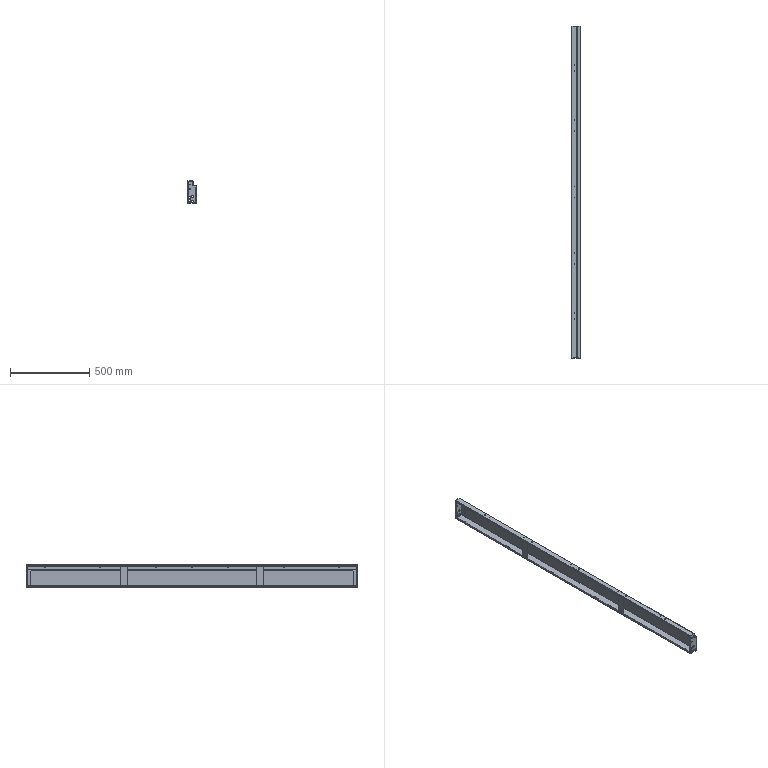Part | SolidWorks | features MirrorCompFeat 2, ReferencePattern 2 | 5 solids | 222 faces | box 58 x 2100 x 140 mm | volume 731344 mm3 | plane 122 | cylinder 100 | commonest cylinder face diameters 5 x32 11 x20 9 x18 4.6 x14 2 x10 4.4 x6